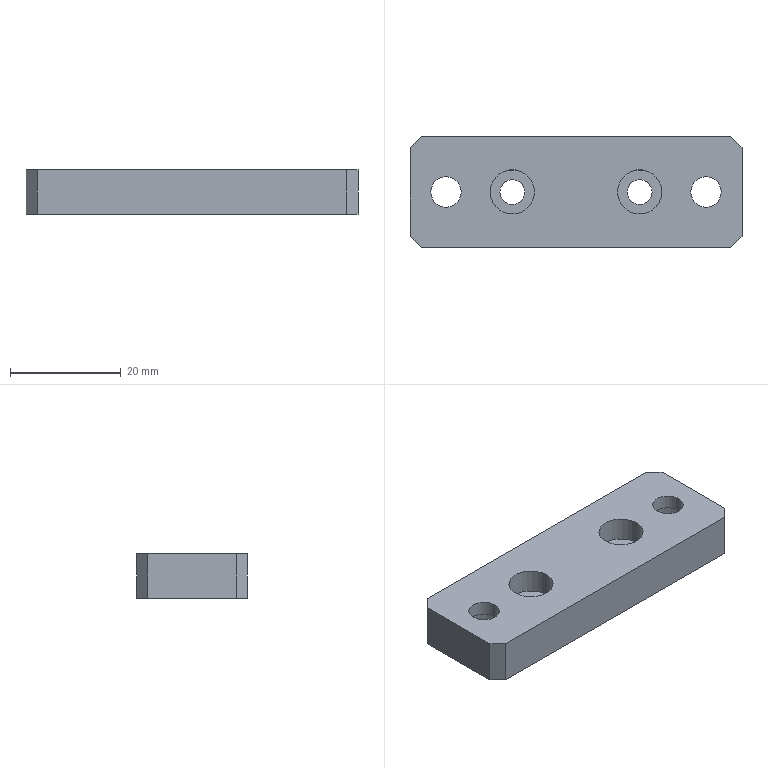Part | SolidWorks | features HoleWzd 2, Chamfer 1, Extrusion 1 | 1 solid | 30 faces | box 60 x 20 x 8 mm | volume 8007 mm3 | cylinder 16 | plane 14 | commonest cylinder face diameters 4.5 x4 5.5 x4 8 x4 10 x4
STEP:
#1=CARTESIAN_POINT('',(11.5,10.,5.4));
#2=VERTEX_POINT('',#1);
#3=CARTESIAN_POINT('',(1.5,10.,5.4));
#4=VERTEX_POINT('',#3);
#5=CARTESIAN_POINT('',(6.5,10.,5.4));
#6=DIRECTION('',(0.,0.,-1.));
#7=DIRECTION('',(-1.,0.,0.));
#8=AXIS2_PLACEMENT_3D('',#5,#6,#7);
#9=CIRCLE('',#8,5.);
#10=EDGE_CURVE('',#2,#4,#9,.T.);
#11=ORIENTED_EDGE('',*,*,#10,.F.);
#12=CARTESIAN_POINT('',(11.5,10.,0.));
#13=VERTEX_POINT('',#12);
#14=CARTESIAN_POINT('',(11.5,10.,0.));
#15=DIRECTION('',(0.,0.,-1.));
#16=VECTOR('',#15,1000.);
#17=LINE('',#14,#16);
#18=EDGE_CURVE('',#2,#13,#17,.T.);
#19=ORIENTED_EDGE('',*,*,#18,.T.);
#20=CARTESIAN_POINT('',(1.5,10.,0.));
#21=VERTEX_POINT('',#20);
#22=CARTESIAN_POINT('',(6.5,10.,0.));
#23=DIRECTION('',(0.,0.,-1.));
#24=DIRECTION('',(-1.,0.,0.));
#25=AXIS2_PLACEMENT_3D('',#22,#23,#24);
#26=CIRCLE('',#25,5.);
#27=EDGE_CURVE('',#13,#21,#26,.T.);
#28=ORIENTED_EDGE('',*,*,#27,.T.);
#29=CARTESIAN_POINT('',(1.5,10.,0.));
#30=DIRECTION('',(0.,0.,-1.));
#31=VECTOR('',#30,1000.);
#32=LINE('',#29,#31);
#33=EDGE_CURVE('',#4,#21,#32,.T.);
#34=ORIENTED_EDGE('',*,*,#33,.F.);
#35=EDGE_LOOP('',(#11,#19,#28,#34));
#36=FACE_OUTER_BOUND('',#35,.T.);
#37=CARTESIAN_POINT('',(6.5,10.,0.));
#38=DIRECTION('',(0.,0.,-1.));
#39=DIRECTION('',(-1.,0.,0.));
#40=AXIS2_PLACEMENT_3D('',#37,#38,#39);
#41=CYLINDRICAL_SURFACE('',#40,5.);
#42=ADVANCED_FACE('',(#36),#41,.F.);
#43=CARTESIAN_POINT('',(9.25,10.,8.));
#44=VERTEX_POINT('',#43);
#45=CARTESIAN_POINT('',(3.75,10.,8.));
#46=VERTEX_POINT('',#45);
#47=CARTESIAN_POINT('',(6.5,10.,8.));
#48=DIRECTION('',(0.,0.,-1.));
#49=DIRECTION('',(-1.,0.,0.));
#50=AXIS2_PLACEMENT_3D('',#47,#48,#49);
#51=CIRCLE('',#50,2.75);
#52=EDGE_CURVE('',#44,#46,#51,.T.);
#53=ORIENTED_EDGE('',*,*,#52,.F.);
#54=CARTESIAN_POINT('',(9.25,10.,5.4));
#55=VERTEX_POINT('',#54);
#56=CARTESIAN_POINT('',(9.25,10.,0.));
#57=DIRECTION('',(0.,0.,-1.));
#58=VECTOR('',#57,1000.);
#59=LINE('',#56,#58);
#60=EDGE_CURVE('',#44,#55,#59,.T.);
#61=ORIENTED_EDGE('',*,*,#60,.T.);
#62=CARTESIAN_POINT('',(3.75,10.,5.4));
#63=VERTEX_POINT('',#62);
#64=CARTESIAN_POINT('',(6.5,10.,5.4));
#65=DIRECTION('',(0.,0.,-1.));
#66=DIRECTION('',(-1.,0.,0.));
#67=AXIS2_PLACEMENT_3D('',#64,#65,#66);
#68=CIRCLE('',#67,2.75);
#69=EDGE_CURVE('',#55,#63,#68,.T.);
#70=ORIENTED_EDGE('',*,*,#69,.T.);
#71=CARTESIAN_POINT('',(3.75,10.,0.));
#72=DIRECTION('',(0.,0.,-1.));
#73=VECTOR('',#72,1000.);
#74=LINE('',#71,#73);
#75=EDGE_CURVE('',#46,#63,#74,.T.);
#76=ORIENTED_EDGE('',*,*,#75,.F.);
#77=EDGE_LOOP('',(#53,#61,#70,#76));
#78=FACE_OUTER_BOUND('',#77,.T.);
#79=CARTESIAN_POINT('',(6.5,10.,0.));
#80=DIRECTION('',(0.,0.,-1.));
#81=DIRECTION('',(-1.,0.,0.));
#82=AXIS2_PLACEMENT_3D('',#79,#80,#81);
#83=CYLINDRICAL_SURFACE('',#82,2.75);
#84=ADVANCED_FACE('',(#78),#83,.F.);
#85=CARTESIAN_POINT('',(58.5,10.,5.4));
#86=VERTEX_POINT('',#85);
#87=CARTESIAN_POINT('',(48.5,10.,5.4));
#88=VERTEX_POINT('',#87);
#89=CARTESIAN_POINT('',(53.5,10.,5.4));
#90=DIRECTION('',(0.,0.,-1.));
#91=DIRECTION('',(-1.,0.,0.));
#92=AXIS2_PLACEMENT_3D('',#89,#90,#91);
#93=CIRCLE('',#92,5.);
#94=EDGE_CURVE('',#86,#88,#93,.T.);
#95=ORIENTED_EDGE('',*,*,#94,.F.);
#96=CARTESIAN_POINT('',(58.5,10.,0.));
#97=VERTEX_POINT('',#96);
#98=CARTESIAN_POINT('',(58.5,10.,0.));
#99=DIRECTION('',(0.,0.,-1.));
#100=VECTOR('',#99,1000.);
#101=LINE('',#98,#100);
#102=EDGE_CURVE('',#86,#97,#101,.T.);
#103=ORIENTED_EDGE('',*,*,#102,.T.);
#104=CARTESIAN_POINT('',(48.5,10.,0.));
#105=VERTEX_POINT('',#104);
#106=CARTESIAN_POINT('',(53.5,10.,0.));
#107=DIRECTION('',(0.,0.,-1.));
#108=DIRECTION('',(-1.,0.,0.));
#109=AXIS2_PLACEMENT_3D('',#106,#107,#108);
#110=CIRCLE('',#109,5.);
#111=EDGE_CURVE('',#97,#105,#110,.T.);
#112=ORIENTED_EDGE('',*,*,#111,.T.);
#113=CARTESIAN_POINT('',(48.5,10.,0.));
#114=DIRECTION('',(0.,0.,-1.));
#115=VECTOR('',#114,1000.);
#116=LINE('',#113,#115);
#117=EDGE_CURVE('',#88,#105,#116,.T.);
#118=ORIENTED_EDGE('',*,*,#117,.F.);
#119=EDGE_LOOP('',(#95,#103,#112,#118));
#120=FACE_OUTER_BOUND('',#119,.T.);
#121=CARTESIAN_POINT('',(53.5,10.,0.));
#122=DIRECTION('',(0.,0.,-1.));
#123=DIRECTION('',(-1.,0.,0.));
#124=AXIS2_PLACEMENT_3D('',#121,#122,#123);
#125=CYLINDRICAL_SURFACE('',#124,5.);
#126=ADVANCED_FACE('',(#120),#125,.F.);
#127=CARTESIAN_POINT('',(56.25,10.,8.));
#128=VERTEX_POINT('',#127);
#129=CARTESIAN_POINT('',(50.75,10.,8.));
#130=VERTEX_POINT('',#129);
#131=CARTESIAN_POINT('',(53.5,10.,8.));
#132=DIRECTION('',(0.,0.,-1.));
#133=DIRECTION('',(-1.,0.,0.));
#134=AXIS2_PLACEMENT_3D('',#131,#132,#133);
#135=CIRCLE('',#134,2.75);
#136=EDGE_CURVE('',#128,#130,#135,.T.);
#137=ORIENTED_EDGE('',*,*,#136,.F.);
#138=CARTESIAN_POINT('',(56.25,10.,5.4));
#139=VERTEX_POINT('',#138);
#140=CARTESIAN_POINT('',(56.25,10.,0.));
#141=DIRECTION('',(0.,0.,-1.));
#142=VECTOR('',#141,1000.);
#143=LINE('',#140,#142);
#144=EDGE_CURVE('',#128,#139,#143,.T.);
#145=ORIENTED_EDGE('',*,*,#144,.T.);
#146=CARTESIAN_POINT('',(50.75,10.,5.4));
#147=VERTEX_POINT('',#146);
#148=CARTESIAN_POINT('',(53.5,10.,5.4));
#149=DIRECTION('',(0.,0.,-1.));
#150=DIRECTION('',(-1.,0.,0.));
#151=AXIS2_PLACEMENT_3D('',#148,#149,#150);
#152=CIRCLE('',#151,2.75);
#153=EDGE_CURVE('',#139,#147,#152,.T.);
#154=ORIENTED_EDGE('',*,*,#153,.T.);
#155=CARTESIAN_POINT('',(50.75,10.,0.));
#156=DIRECTION('',(0.,0.,-1.));
#157=VECTOR('',#156,1000.);
#158=LINE('',#155,#157);
#159=EDGE_CURVE('',#130,#147,#158,.T.);
#160=ORIENTED_EDGE('',*,*,#159,.F.);
#161=EDGE_LOOP('',(#137,#145,#154,#160));
#162=FACE_OUTER_BOUND('',#161,.T.);
#163=CARTESIAN_POINT('',(53.5,10.,0.));
#164=DIRECTION('',(0.,0.,-1.));
#165=DIRECTION('',(-1.,0.,0.));
#166=AXIS2_PLACEMENT_3D('',#163,#164,#165);
#167=CYLINDRICAL_SURFACE('',#166,2.75);
#168=ADVANCED_FACE('',(#162),#167,.F.);
#169=CARTESIAN_POINT('',(14.5,10.,3.6));
#170=VERTEX_POINT('',#169);
#171=CARTESIAN_POINT('',(22.5,10.,3.6));
#172=VERTEX_POINT('',#171);
#173=CARTESIAN_POINT('',(18.5,10.,3.6));
#174=DIRECTION('',(0.,0.,1.));
#175=DIRECTION('',(1.,0.,0.));
#176=AXIS2_PLACEMENT_3D('',#173,#174,#175);
#177=CIRCLE('',#176,4.);
#178=EDGE_CURVE('',#170,#172,#177,.T.);
#179=ORIENTED_EDGE('',*,*,#178,.F.);
#180=CARTESIAN_POINT('',(14.5,10.,8.));
#181=VERTEX_POINT('',#180);
#182=CARTESIAN_POINT('',(14.5,10.,8.));
#183=DIRECTION('',(0.,0.,1.));
#184=VECTOR('',#183,1000.);
#185=LINE('',#182,#184);
#186=EDGE_CURVE('',#170,#181,#185,.T.);
#187=ORIENTED_EDGE('',*,*,#186,.T.);
#188=CARTESIAN_POINT('',(22.5,10.,8.));
#189=VERTEX_POINT('',#188);
#190=CARTESIAN_POINT('',(18.5,10.,8.));
#191=DIRECTION('',(0.,0.,1.));
#192=DIRECTION('',(1.,0.,0.));
#193=AXIS2_PLACEMENT_3D('',#190,#191,#192);
#194=CIRCLE('',#193,4.);
#195=EDGE_CURVE('',#181,#189,#194,.T.);
#196=ORIENTED_EDGE('',*,*,#195,.T.);
#197=CARTESIAN_POINT('',(22.5,10.,8.));
#198=DIRECTION('',(0.,0.,1.));
#199=VECTOR('',#198,1000.);
#200=LINE('',#197,#199);
#201=EDGE_CURVE('',#172,#189,#200,.T.);
#202=ORIENTED_EDGE('',*,*,#201,.F.);
#203=EDGE_LOOP('',(#179,#187,#196,#202));
#204=FACE_OUTER_BOUND('',#203,.T.);
#205=CARTESIAN_POINT('',(18.5,10.,8.));
#206=DIRECTION('',(0.,0.,1.));
#207=DIRECTION('',(1.,0.,0.));
#208=AXIS2_PLACEMENT_3D('',#205,#206,#207);
#209=CYLINDRICAL_SURFACE('',#208,4.);
#210=ADVANCED_FACE('',(#204),#209,.F.);
#211=CARTESIAN_POINT('',(16.25,10.,0.));
#212=VERTEX_POINT('',#211);
#213=CARTESIAN_POINT('',(20.75,10.,0.));
#214=VERTEX_POINT('',#213);
#215=CARTESIAN_POINT('',(18.5,10.,0.));
#216=DIRECTION('',(0.,0.,1.));
#217=DIRECTION('',(1.,0.,0.));
#218=AXIS2_PLACEMENT_3D('',#215,#216,#217);
#219=CIRCLE('',#218,2.25);
#220=EDGE_CURVE('',#212,#214,#219,.T.);
#221=ORIENTED_EDGE('',*,*,#220,.F.);
#222=CARTESIAN_POINT('',(16.25,10.,3.6));
#223=VERTEX_POINT('',#222);
#224=CARTESIAN_POINT('',(16.25,10.,8.));
#225=DIRECTION('',(0.,0.,1.));
#226=VECTOR('',#225,1000.);
#227=LINE('',#224,#226);
#228=EDGE_CURVE('',#212,#223,#227,.T.);
#229=ORIENTED_EDGE('',*,*,#228,.T.);
#230=CARTESIAN_POINT('',(20.75,10.,3.6));
#231=VERTEX_POINT('',#230);
#232=CARTESIAN_POINT('',(18.5,10.,3.6));
#233=DIRECTION('',(0.,0.,1.));
#234=DIRECTION('',(1.,0.,0.));
#235=AXIS2_PLACEMENT_3D('',#232,#233,#234);
#236=CIRCLE('',#235,2.25);
#237=EDGE_CURVE('',#223,#231,#236,.T.);
#238=ORIENTED_EDGE('',*,*,#237,.T.);
#239=CARTESIAN_POINT('',(20.75,10.,8.));
#240=DIRECTION('',(0.,0.,1.));
#241=VECTOR('',#240,1000.);
#242=LINE('',#239,#241);
#243=EDGE_CURVE('',#214,#231,#242,.T.);
#244=ORIENTED_EDGE('',*,*,#243,.F.);
#245=EDGE_LOOP('',(#221,#229,#238,#244));
#246=FACE_OUTER_BOUND('',#245,.T.);
#247=CARTESIAN_POINT('',(18.5,10.,8.));
#248=DIRECTION('',(0.,0.,1.));
#249=DIRECTION('',(1.,0.,0.));
#250=AXIS2_PLACEMENT_3D('',#247,#248,#249);
#251=CYLINDRICAL_SURFACE('',#250,2.25);
#252=ADVANCED_FACE('',(#246),#251,.F.);
#253=CARTESIAN_POINT('',(37.5,10.,3.6));
#254=VERTEX_POINT('',#253);
#255=CARTESIAN_POINT('',(45.5,10.,3.6));
#256=VERTEX_POINT('',#255);
#257=CARTESIAN_POINT('',(41.5,10.,3.6));
#258=DIRECTION('',(0.,0.,1.));
#259=DIRECTION('',(1.,0.,0.));
#260=AXIS2_PLACEMENT_3D('',#257,#258,#259);
#261=CIRCLE('',#260,4.);
#262=EDGE_CURVE('',#254,#256,#261,.T.);
#263=ORIENTED_EDGE('',*,*,#262,.F.);
#264=CARTESIAN_POINT('',(37.5,10.,8.));
#265=VERTEX_POINT('',#264);
#266=CARTESIAN_POINT('',(37.5,10.,8.));
#267=DIRECTION('',(0.,0.,1.));
#268=VECTOR('',#267,1000.);
#269=LINE('',#266,#268);
#270=EDGE_CURVE('',#254,#265,#269,.T.);
#271=ORIENTED_EDGE('',*,*,#270,.T.);
#272=CARTESIAN_POINT('',(45.5,10.,8.));
#273=VERTEX_POINT('',#272);
#274=CARTESIAN_POINT('',(41.5,10.,8.));
#275=DIRECTION('',(0.,0.,1.));
#276=DIRECTION('',(1.,0.,0.));
#277=AXIS2_PLACEMENT_3D('',#274,#275,#276);
#278=CIRCLE('',#277,4.);
#279=EDGE_CURVE('',#265,#273,#278,.T.);
#280=ORIENTED_EDGE('',*,*,#279,.T.);
#281=CARTESIAN_POINT('',(45.5,10.,8.));
#282=DIRECTION('',(0.,0.,1.));
#283=VECTOR('',#282,1000.);
#284=LINE('',#281,#283);
#285=EDGE_CURVE('',#256,#273,#284,.T.);
#286=ORIENTED_EDGE('',*,*,#285,.F.);
#287=EDGE_LOOP('',(#263,#271,#280,#286));
#288=FACE_OUTER_BOUND('',#287,.T.);
#289=CARTESIAN_POINT('',(41.5,10.,8.));
#290=DIRECTION('',(0.,0.,1.));
#291=DIRECTION('',(1.,0.,0.));
#292=AXIS2_PLACEMENT_3D('',#289,#290,#291);
#293=CYLINDRICAL_SURFACE('',#292,4.);
#294=ADVANCED_FACE('',(#288),#293,.F.);
#295=CARTESIAN_POINT('',(39.25,10.,0.));
#296=VERTEX_POINT('',#295);
#297=CARTESIAN_POINT('',(43.75,10.,0.));
#298=VERTEX_POINT('',#297);
#299=CARTESIAN_POINT('',(41.5,10.,0.));
#300=DIRECTION('',(0.,0.,1.));
#301=DIRECTION('',(1.,0.,0.));
#302=AXIS2_PLACEMENT_3D('',#299,#300,#301);
#303=CIRCLE('',#302,2.25);
#304=EDGE_CURVE('',#296,#298,#303,.T.);
#305=ORIENTED_EDGE('',*,*,#304,.F.);
#306=CARTESIAN_POINT('',(39.25,10.,3.6));
#307=VERTEX_POINT('',#306);
#308=CARTESIAN_POINT('',(39.25,10.,8.));
#309=DIRECTION('',(0.,0.,1.));
#310=VECTOR('',#309,1000.);
#311=LINE('',#308,#310);
#312=EDGE_CURVE('',#296,#307,#311,.T.);
#313=ORIENTED_EDGE('',*,*,#312,.T.);
#314=CARTESIAN_POINT('',(43.75,10.,3.6));
#315=VERTEX_POINT('',#314);
#316=CARTESIAN_POINT('',(41.5,10.,3.6));
#317=DIRECTION('',(0.,0.,1.));
#318=DIRECTION('',(1.,0.,0.));
#319=AXIS2_PLACEMENT_3D('',#316,#317,#318);
#320=CIRCLE('',#319,2.25);
#321=EDGE_CURVE('',#307,#315,#320,.T.);
#322=ORIENTED_EDGE('',*,*,#321,.T.);
#323=CARTESIAN_POINT('',(43.75,10.,8.));
#324=DIRECTION('',(0.,0.,1.));
#325=VECTOR('',#324,1000.);
#326=LINE('',#323,#325);
#327=EDGE_CURVE('',#298,#315,#326,.T.);
#328=ORIENTED_EDGE('',*,*,#327,.F.);
#329=EDGE_LOOP('',(#305,#313,#322,#328));
#330=FACE_OUTER_BOUND('',#329,.T.);
#331=CARTESIAN_POINT('',(41.5,10.,8.));
#332=DIRECTION('',(0.,0.,1.));
#333=DIRECTION('',(1.,0.,0.));
#334=AXIS2_PLACEMENT_3D('',#331,#332,#333);
#335=CYLINDRICAL_SURFACE('',#334,2.25);
#336=ADVANCED_FACE('',(#330),#335,.F.);
#337=CARTESIAN_POINT('',(0.,18.,8.));
#338=VERTEX_POINT('',#337);
#339=CARTESIAN_POINT('',(0.,2.,8.));
#340=VERTEX_POINT('',#339);
#341=CARTESIAN_POINT('',(0.,0.,8.));
#342=DIRECTION('',(0.,-1.,0.));
#343=VECTOR('',#342,1000.);
#344=LINE('',#341,#343);
#345=EDGE_CURVE('',#338,#340,#344,.T.);
#346=ORIENTED_EDGE('',*,*,#345,.F.);
#347=CARTESIAN_POINT('',(0.,18.,0.));
#348=VERTEX_POINT('',#347);
#349=CARTESIAN_POINT('',(0.,18.,8.));
#350=DIRECTION('',(0.,0.,-1.));
#351=VECTOR('',#350,1000.);
#352=LINE('',#349,#351);
#353=EDGE_CURVE('',#338,#348,#352,.T.);
#354=ORIENTED_EDGE('',*,*,#353,.T.);
#355=CARTESIAN_POINT('',(0.,2.,0.));
#356=VERTEX_POINT('',#355);
#357=CARTESIAN_POINT('',(0.,0.,0.));
#358=DIRECTION('',(0.,-1.,0.));
#359=VECTOR('',#358,1000.);
#360=LINE('',#357,#359);
#361=EDGE_CURVE('',#348,#356,#360,.T.);
#362=ORIENTED_EDGE('',*,*,#361,.T.);
#363=CARTESIAN_POINT('',(0.,2.,8.));
#364=DIRECTION('',(0.,0.,1.));
#365=VECTOR('',#364,1000.);
#366=LINE('',#363,#365);
#367=EDGE_CURVE('',#356,#340,#366,.T.);
#368=ORIENTED_EDGE('',*,*,#367,.T.);
#369=EDGE_LOOP('',(#346,#354,#362,#368));
#370=FACE_OUTER_BOUND('',#369,.T.);
#371=CARTESIAN_POINT('',(0.,0.,8.));
#372=DIRECTION('',(1.,0.,0.));
#373=DIRECTION('',(0.,0.,-1.));
#374=AXIS2_PLACEMENT_3D('',#371,#372,#373);
#375=PLANE('',#374);
#376=ADVANCED_FACE('',(#370),#375,.F.);
#377=CARTESIAN_POINT('',(2.,0.,0.));
#378=VERTEX_POINT('',#377);
#379=CARTESIAN_POINT('',(58.,0.,0.));
#380=VERTEX_POINT('',#379);
#381=CARTESIAN_POINT('',(0.,0.,0.));
#382=DIRECTION('',(1.,0.,0.));
#383=VECTOR('',#382,1000.);
#384=LINE('',#381,#383);
#385=EDGE_CURVE('',#378,#380,#384,.T.);
#386=ORIENTED_EDGE('',*,*,#385,.T.);
#387=CARTESIAN_POINT('',(58.,0.,8.));
#388=VERTEX_POINT('',#387);
#389=CARTESIAN_POINT('',(58.,0.,8.));
#390=DIRECTION('',(0.,0.,1.));
#391=VECTOR('',#390,1000.);
#392=LINE('',#389,#391);
#393=EDGE_CURVE('',#380,#388,#392,.T.);
#394=ORIENTED_EDGE('',*,*,#393,.T.);
#395=CARTESIAN_POINT('',(2.,0.,8.));
#396=VERTEX_POINT('',#395);
#397=CARTESIAN_POINT('',(0.,0.,8.));
#398=DIRECTION('',(1.,0.,0.));
#399=VECTOR('',#398,1000.);
#400=LINE('',#397,#399);
#401=EDGE_CURVE('',#396,#388,#400,.T.);
#402=ORIENTED_EDGE('',*,*,#401,.F.);
#403=CARTESIAN_POINT('',(2.,0.,8.));
#404=DIRECTION('',(0.,0.,-1.));
#405=VECTOR('',#404,1000.);
#406=LINE('',#403,#405);
#407=EDGE_CURVE('',#396,#378,#406,.T.);
#408=ORIENTED_EDGE('',*,*,#407,.T.);
#409=EDGE_LOOP('',(#386,#394,#402,#408));
#410=FACE_OUTER_BOUND('',#409,.T.);
#411=CARTESIAN_POINT('',(0.,0.,8.));
#412=DIRECTION('',(0.,1.,0.));
#413=DIRECTION('',(0.,0.,1.));
#414=AXIS2_PLACEMENT_3D('',#411,#412,#413);
#415=PLANE('',#414);
#416=ADVANCED_FACE('',(#410),#415,.F.);
#417=CARTESIAN_POINT('',(60.,2.,0.));
#418=VERTEX_POINT('',#417);
#419=CARTESIAN_POINT('',(60.,18.,0.));
#420=VERTEX_POINT('',#419);
#421=CARTESIAN_POINT('',(60.,0.,0.));
#422=DIRECTION('',(0.,1.,0.));
#423=VECTOR('',#422,1000.);
#424=LINE('',#421,#423);
#425=EDGE_CURVE('',#418,#420,#424,.T.);
#426=ORIENTED_EDGE('',*,*,#425,.T.);
#427=CARTESIAN_POINT('',(60.,18.,8.));
#428=VERTEX_POINT('',#427);
#429=CARTESIAN_POINT('',(60.,18.,8.));
#430=DIRECTION('',(0.,0.,1.));
#431=VECTOR('',#430,1000.);
#432=LINE('',#429,#431);
#433=EDGE_CURVE('',#420,#428,#432,.T.);
#434=ORIENTED_EDGE('',*,*,#433,.T.);
#435=CARTESIAN_POINT('',(60.,2.,8.));
#436=VERTEX_POINT('',#435);
#437=CARTESIAN_POINT('',(60.,0.,8.));
#438=DIRECTION('',(0.,1.,0.));
#439=VECTOR('',#438,1000.);
#440=LINE('',#437,#439);
#441=EDGE_CURVE('',#436,#428,#440,.T.);
#442=ORIENTED_EDGE('',*,*,#441,.F.);
#443=CARTESIAN_POINT('',(60.,2.,8.));
#444=DIRECTION('',(0.,0.,-1.));
#445=VECTOR('',#444,1000.);
#446=LINE('',#443,#445);
#447=EDGE_CURVE('',#436,#418,#446,.T.);
#448=ORIENTED_EDGE('',*,*,#447,.T.);
#449=EDGE_LOOP('',(#426,#434,#442,#448));
#450=FACE_OUTER_BOUND('',#449,.T.);
#451=CARTESIAN_POINT('',(60.,0.,8.));
#452=DIRECTION('',(-1.,0.,0.));
#453=DIRECTION('',(0.,0.,1.));
#454=AXIS2_PLACEMENT_3D('',#451,#452,#453);
#455=PLANE('',#454);
#456=ADVANCED_FACE('',(#450),#455,.F.);
#457=CARTESIAN_POINT('',(58.,20.,8.));
#458=VERTEX_POINT('',#457);
#459=CARTESIAN_POINT('',(2.,20.,8.));
#460=VERTEX_POINT('',#459);
#461=CARTESIAN_POINT('',(0.,20.,8.));
#462=DIRECTION('',(-1.,0.,0.));
#463=VECTOR('',#462,1000.);
#464=LINE('',#461,#463);
#465=EDGE_CURVE('',#458,#460,#464,.T.);
#466=ORIENTED_EDGE('',*,*,#465,.F.);
#467=CARTESIAN_POINT('',(58.,20.,0.));
#468=VERTEX_POINT('',#467);
#469=CARTESIAN_POINT('',(58.,20.,8.));
#470=DIRECTION('',(0.,0.,-1.));
#471=VECTOR('',#470,1000.);
#472=LINE('',#469,#471);
#473=EDGE_CURVE('',#458,#468,#472,.T.);
#474=ORIENTED_EDGE('',*,*,#473,.T.);
#475=CARTESIAN_POINT('',(2.,20.,0.));
#476=VERTEX_POINT('',#475);
#477=CARTESIAN_POINT('',(0.,20.,0.));
#478=DIRECTION('',(-1.,0.,0.));
#479=VECTOR('',#478,1000.);
#480=LINE('',#477,#479);
#481=EDGE_CURVE('',#468,#476,#480,.T.);
#482=ORIENTED_EDGE('',*,*,#481,.T.);
#483=CARTESIAN_POINT('',(2.,20.,8.));
#484=DIRECTION('',(0.,0.,1.));
#485=VECTOR('',#484,1000.);
#486=LINE('',#483,#485);
#487=EDGE_CURVE('',#476,#460,#486,.T.);
#488=ORIENTED_EDGE('',*,*,#487,.T.);
#489=EDGE_LOOP('',(#466,#474,#482,#488));
#490=FACE_OUTER_BOUND('',#489,.T.);
#491=CARTESIAN_POINT('',(0.,20.,8.));
#492=DIRECTION('',(0.,-1.,0.));
#493=DIRECTION('',(0.,0.,-1.));
#494=AXIS2_PLACEMENT_3D('',#491,#492,#493);
#495=PLANE('',#494);
#496=ADVANCED_FACE('',(#490),#495,.F.);
#497=CARTESIAN_POINT('',(6.5,10.,8.));
#498=DIRECTION('',(0.,0.,-1.));
#499=DIRECTION('',(-1.,0.,0.));
#500=AXIS2_PLACEMENT_3D('',#497,#498,#499);
#501=CIRCLE('',#500,2.75);
#502=EDGE_CURVE('',#46,#44,#501,.T.);
#503=ORIENTED_EDGE('',*,*,#502,.T.);
#504=ORIENTED_EDGE('',*,*,#52,.T.);
#505=EDGE_LOOP('',(#503,#504));
#506=FACE_BOUND('',#505,.T.);
#507=CARTESIAN_POINT('',(53.5,10.,8.));
#508=DIRECTION('',(0.,0.,-1.));
#509=DIRECTION('',(-1.,0.,0.));
#510=AXIS2_PLACEMENT_3D('',#507,#508,#509);
#511=CIRCLE('',#510,2.75);
#512=EDGE_CURVE('',#130,#128,#511,.T.);
#513=ORIENTED_EDGE('',*,*,#512,.T.);
#514=ORIENTED_EDGE('',*,*,#136,.T.);
#515=EDGE_LOOP('',(#513,#514));
#516=FACE_BOUND('',#515,.T.);
#517=CARTESIAN_POINT('',(18.5,10.,8.));
#518=DIRECTION('',(0.,0.,1.));
#519=DIRECTION('',(1.,0.,0.));
#520=AXIS2_PLACEMENT_3D('',#517,#518,#519);
#521=CIRCLE('',#520,4.);
#522=EDGE_CURVE('',#189,#181,#521,.T.);
#523=ORIENTED_EDGE('',*,*,#522,.F.);
#524=ORIENTED_EDGE('',*,*,#195,.F.);
#525=EDGE_LOOP('',(#523,#524));
#526=FACE_BOUND('',#525,.T.);
#527=CARTESIAN_POINT('',(41.5,10.,8.));
#528=DIRECTION('',(0.,0.,1.));
#529=DIRECTION('',(1.,0.,0.));
#530=AXIS2_PLACEMENT_3D('',#527,#528,#529);
#531=CIRCLE('',#530,4.);
#532=EDGE_CURVE('',#273,#265,#531,.T.);
#533=ORIENTED_EDGE('',*,*,#532,.F.);
#534=ORIENTED_EDGE('',*,*,#279,.F.);
#535=EDGE_LOOP('',(#533,#534));
#536=FACE_BOUND('',#535,.T.);
#537=ORIENTED_EDGE('',*,*,#441,.T.);
#538=CARTESIAN_POINT('',(58.,20.,8.));
#539=DIRECTION('',(-0.7071,0.7071,0.));
#540=VECTOR('',#539,1000.);
#541=LINE('',#538,#540);
#542=EDGE_CURVE('',#428,#458,#541,.T.);
#543=ORIENTED_EDGE('',*,*,#542,.T.);
#544=ORIENTED_EDGE('',*,*,#465,.T.);
#545=CARTESIAN_POINT('',(0.,18.,8.));
#546=DIRECTION('',(-0.7071,-0.7071,0.));
#547=VECTOR('',#546,1000.);
#548=LINE('',#545,#547);
#549=EDGE_CURVE('',#460,#338,#548,.T.);
#550=ORIENTED_EDGE('',*,*,#549,.T.);
#551=ORIENTED_EDGE('',*,*,#345,.T.);
#552=CARTESIAN_POINT('',(2.,0.,8.));
#553=DIRECTION('',(0.7071,-0.7071,0.));
#554=VECTOR('',#553,1000.);
#555=LINE('',#552,#554);
#556=EDGE_CURVE('',#340,#396,#555,.T.);
#557=ORIENTED_EDGE('',*,*,#556,.T.);
#558=ORIENTED_EDGE('',*,*,#401,.T.);
#559=CARTESIAN_POINT('',(60.,2.,8.));
#560=DIRECTION('',(0.7071,0.7071,0.));
#561=VECTOR('',#560,1000.);
#562=LINE('',#559,#561);
#563=EDGE_CURVE('',#388,#436,#562,.T.);
#564=ORIENTED_EDGE('',*,*,#563,.T.);
#565=EDGE_LOOP('',(#537,#543,#544,#550,#551,#557,#558,#564));
#566=FACE_OUTER_BOUND('',#565,.T.);
#567=CARTESIAN_POINT('',(0.,0.,8.));
#568=DIRECTION('',(0.,0.,-1.));
#569=DIRECTION('',(-1.,0.,0.));
#570=AXIS2_PLACEMENT_3D('',#567,#568,#569);
#571=PLANE('',#570);
#572=ADVANCED_FACE('',(#506,#516,#526,#536,#566),#571,.F.);
#573=CARTESIAN_POINT('',(6.5,10.,0.));
#574=DIRECTION('',(0.,0.,-1.));
#575=DIRECTION('',(-1.,0.,0.));
#576=AXIS2_PLACEMENT_3D('',#573,#574,#575);
#577=CIRCLE('',#576,5.);
#578=EDGE_CURVE('',#21,#13,#577,.T.);
#579=ORIENTED_EDGE('',*,*,#578,.F.);
#580=ORIENTED_EDGE('',*,*,#27,.F.);
#581=EDGE_LOOP('',(#579,#580));
#582=FACE_BOUND('',#581,.T.);
#583=CARTESIAN_POINT('',(53.5,10.,0.));
#584=DIRECTION('',(0.,0.,-1.));
#585=DIRECTION('',(-1.,0.,0.));
#586=AXIS2_PLACEMENT_3D('',#583,#584,#585);
#587=CIRCLE('',#586,5.);
#588=EDGE_CURVE('',#105,#97,#587,.T.);
#589=ORIENTED_EDGE('',*,*,#588,.F.);
#590=ORIENTED_EDGE('',*,*,#111,.F.);
#591=EDGE_LOOP('',(#589,#590));
#592=FACE_BOUND('',#591,.T.);
#593=CARTESIAN_POINT('',(18.5,10.,0.));
#594=DIRECTION('',(0.,0.,1.));
#595=DIRECTION('',(1.,0.,0.));
#596=AXIS2_PLACEMENT_3D('',#593,#594,#595);
#597=CIRCLE('',#596,2.25);
#598=EDGE_CURVE('',#214,#212,#597,.T.);
#599=ORIENTED_EDGE('',*,*,#598,.T.);
#600=ORIENTED_EDGE('',*,*,#220,.T.);
#601=EDGE_LOOP('',(#599,#600));
#602=FACE_BOUND('',#601,.T.);
#603=CARTESIAN_POINT('',(41.5,10.,0.));
#604=DIRECTION('',(0.,0.,1.));
#605=DIRECTION('',(1.,0.,0.));
#606=AXIS2_PLACEMENT_3D('',#603,#604,#605);
#607=CIRCLE('',#606,2.25);
#608=EDGE_CURVE('',#298,#296,#607,.T.);
#609=ORIENTED_EDGE('',*,*,#608,.T.);
#610=ORIENTED_EDGE('',*,*,#304,.T.);
#611=EDGE_LOOP('',(#609,#610));
#612=FACE_BOUND('',#611,.T.);
#613=ORIENTED_EDGE('',*,*,#481,.F.);
#614=CARTESIAN_POINT('',(39.,39.,0.));
#615=DIRECTION('',(0.7071,-0.7071,0.));
#616=VECTOR('',#615,1000.);
#617=LINE('',#614,#616);
#618=EDGE_CURVE('',#468,#420,#617,.T.);
#619=ORIENTED_EDGE('',*,*,#618,.T.);
#620=ORIENTED_EDGE('',*,*,#425,.F.);
#621=CARTESIAN_POINT('',(29.,-29.,0.));
#622=DIRECTION('',(-0.7071,-0.7071,0.));
#623=VECTOR('',#622,1000.);
#624=LINE('',#621,#623);
#625=EDGE_CURVE('',#418,#380,#624,.T.);
#626=ORIENTED_EDGE('',*,*,#625,.T.);
#627=ORIENTED_EDGE('',*,*,#385,.F.);
#628=CARTESIAN_POINT('',(1.,1.,0.));
#629=DIRECTION('',(-0.7071,0.7071,0.));
#630=VECTOR('',#629,1000.);
#631=LINE('',#628,#630);
#632=EDGE_CURVE('',#378,#356,#631,.T.);
#633=ORIENTED_EDGE('',*,*,#632,.T.);
#634=ORIENTED_EDGE('',*,*,#361,.F.);
#635=CARTESIAN_POINT('',(-9.,9.,0.));
#636=DIRECTION('',(0.7071,0.7071,0.));
#637=VECTOR('',#636,1000.);
#638=LINE('',#635,#637);
#639=EDGE_CURVE('',#348,#476,#638,.T.);
#640=ORIENTED_EDGE('',*,*,#639,.T.);
#641=EDGE_LOOP('',(#613,#619,#620,#626,#627,#633,#634,#640));
#642=FACE_OUTER_BOUND('',#641,.T.);
#643=CARTESIAN_POINT('',(0.,0.,0.));
#644=DIRECTION('',(0.,0.,-1.));
#645=DIRECTION('',(-1.,0.,0.));
#646=AXIS2_PLACEMENT_3D('',#643,#644,#645);
#647=PLANE('',#646);
#648=ADVANCED_FACE('',(#582,#592,#602,#612,#642),#647,.T.);
#649=ORIENTED_EDGE('',*,*,#312,.F.);
#650=ORIENTED_EDGE('',*,*,#608,.F.);
#651=ORIENTED_EDGE('',*,*,#327,.T.);
#652=CARTESIAN_POINT('',(41.5,10.,3.6));
#653=DIRECTION('',(0.,0.,1.));
#654=DIRECTION('',(1.,0.,0.));
#655=AXIS2_PLACEMENT_3D('',#652,#653,#654);
#656=CIRCLE('',#655,2.25);
#657=EDGE_CURVE('',#315,#307,#656,.T.);
#658=ORIENTED_EDGE('',*,*,#657,.T.);
#659=EDGE_LOOP('',(#649,#650,#651,#658));
#660=FACE_OUTER_BOUND('',#659,.T.);
#661=CARTESIAN_POINT('',(41.5,10.,8.));
#662=DIRECTION('',(0.,0.,1.));
#663=DIRECTION('',(1.,0.,0.));
#664=AXIS2_PLACEMENT_3D('',#661,#662,#663);
#665=CYLINDRICAL_SURFACE('',#664,2.25);
#666=ADVANCED_FACE('',(#660),#665,.F.);
#667=ORIENTED_EDGE('',*,*,#657,.F.);
#668=ORIENTED_EDGE('',*,*,#321,.F.);
#669=EDGE_LOOP('',(#667,#668));
#670=FACE_BOUND('',#669,.T.);
#671=CARTESIAN_POINT('',(41.5,10.,3.6));
#672=DIRECTION('',(0.,0.,1.));
#673=DIRECTION('',(1.,0.,0.));
#674=AXIS2_PLACEMENT_3D('',#671,#672,#673);
#675=CIRCLE('',#674,4.);
#676=EDGE_CURVE('',#256,#254,#675,.T.);
#677=ORIENTED_EDGE('',*,*,#676,.T.);
#678=ORIENTED_EDGE('',*,*,#262,.T.);
#679=EDGE_LOOP('',(#677,#678));
#680=FACE_OUTER_BOUND('',#679,.T.);
#681=CARTESIAN_POINT('',(43.75,10.,3.6));
#682=DIRECTION('',(0.,0.,-1.));
#683=DIRECTION('',(-1.,0.,0.));
#684=AXIS2_PLACEMENT_3D('',#681,#682,#683);
#685=PLANE('',#684);
#686=ADVANCED_FACE('',(#670,#680),#685,.F.);
#687=ORIENTED_EDGE('',*,*,#270,.F.);
#688=ORIENTED_EDGE('',*,*,#676,.F.);
#689=ORIENTED_EDGE('',*,*,#285,.T.);
#690=ORIENTED_EDGE('',*,*,#532,.T.);
#691=EDGE_LOOP('',(#687,#688,#689,#690));
#692=FACE_OUTER_BOUND('',#691,.T.);
#693=CARTESIAN_POINT('',(41.5,10.,8.));
#694=DIRECTION('',(0.,0.,1.));
#695=DIRECTION('',(1.,0.,0.));
#696=AXIS2_PLACEMENT_3D('',#693,#694,#695);
#697=CYLINDRICAL_SURFACE('',#696,4.);
#698=ADVANCED_FACE('',(#692),#697,.F.);
#699=ORIENTED_EDGE('',*,*,#228,.F.);
#700=ORIENTED_EDGE('',*,*,#598,.F.);
#701=ORIENTED_EDGE('',*,*,#243,.T.);
#702=CARTESIAN_POINT('',(18.5,10.,3.6));
#703=DIRECTION('',(0.,0.,1.));
#704=DIRECTION('',(1.,0.,0.));
#705=AXIS2_PLACEMENT_3D('',#702,#703,#704);
#706=CIRCLE('',#705,2.25);
#707=EDGE_CURVE('',#231,#223,#706,.T.);
#708=ORIENTED_EDGE('',*,*,#707,.T.);
#709=EDGE_LOOP('',(#699,#700,#701,#708));
#710=FACE_OUTER_BOUND('',#709,.T.);
#711=CARTESIAN_POINT('',(18.5,10.,8.));
#712=DIRECTION('',(0.,0.,1.));
#713=DIRECTION('',(1.,0.,0.));
#714=AXIS2_PLACEMENT_3D('',#711,#712,#713);
#715=CYLINDRICAL_SURFACE('',#714,2.25);
#716=ADVANCED_FACE('',(#710),#715,.F.);
#717=ORIENTED_EDGE('',*,*,#707,.F.);
#718=ORIENTED_EDGE('',*,*,#237,.F.);
#719=EDGE_LOOP('',(#717,#718));
#720=FACE_BOUND('',#719,.T.);
#721=CARTESIAN_POINT('',(18.5,10.,3.6));
#722=DIRECTION('',(0.,0.,1.));
#723=DIRECTION('',(1.,0.,0.));
#724=AXIS2_PLACEMENT_3D('',#721,#722,#723);
#725=CIRCLE('',#724,4.);
#726=EDGE_CURVE('',#172,#170,#725,.T.);
#727=ORIENTED_EDGE('',*,*,#726,.T.);
#728=ORIENTED_EDGE('',*,*,#178,.T.);
#729=EDGE_LOOP('',(#727,#728));
#730=FACE_OUTER_BOUND('',#729,.T.);
#731=CARTESIAN_POINT('',(20.75,10.,3.6));
#732=DIRECTION('',(0.,0.,-1.));
#733=DIRECTION('',(-1.,0.,0.));
#734=AXIS2_PLACEMENT_3D('',#731,#732,#733);
#735=PLANE('',#734);
#736=ADVANCED_FACE('',(#720,#730),#735,.F.);
#737=ORIENTED_EDGE('',*,*,#186,.F.);
#738=ORIENTED_EDGE('',*,*,#726,.F.);
#739=ORIENTED_EDGE('',*,*,#201,.T.);
#740=ORIENTED_EDGE('',*,*,#522,.T.);
#741=EDGE_LOOP('',(#737,#738,#739,#740));
#742=FACE_OUTER_BOUND('',#741,.T.);
#743=CARTESIAN_POINT('',(18.5,10.,8.));
#744=DIRECTION('',(0.,0.,1.));
#745=DIRECTION('',(1.,0.,0.));
#746=AXIS2_PLACEMENT_3D('',#743,#744,#745);
#747=CYLINDRICAL_SURFACE('',#746,4.);
#748=ADVANCED_FACE('',(#742),#747,.F.);
#749=ORIENTED_EDGE('',*,*,#144,.F.);
#750=ORIENTED_EDGE('',*,*,#512,.F.);
#751=ORIENTED_EDGE('',*,*,#159,.T.);
#752=CARTESIAN_POINT('',(53.5,10.,5.4));
#753=DIRECTION('',(0.,0.,-1.));
#754=DIRECTION('',(-1.,0.,0.));
#755=AXIS2_PLACEMENT_3D('',#752,#753,#754);
#756=CIRCLE('',#755,2.75);
#757=EDGE_CURVE('',#147,#139,#756,.T.);
#758=ORIENTED_EDGE('',*,*,#757,.T.);
#759=EDGE_LOOP('',(#749,#750,#751,#758));
#760=FACE_OUTER_BOUND('',#759,.T.);
#761=CARTESIAN_POINT('',(53.5,10.,0.));
#762=DIRECTION('',(0.,0.,-1.));
#763=DIRECTION('',(-1.,0.,0.));
#764=AXIS2_PLACEMENT_3D('',#761,#762,#763);
#765=CYLINDRICAL_SURFACE('',#764,2.75);
#766=ADVANCED_FACE('',(#760),#765,.F.);
#767=ORIENTED_EDGE('',*,*,#757,.F.);
#768=ORIENTED_EDGE('',*,*,#153,.F.);
#769=EDGE_LOOP('',(#767,#768));
#770=FACE_BOUND('',#769,.T.);
#771=CARTESIAN_POINT('',(53.5,10.,5.4));
#772=DIRECTION('',(0.,0.,-1.));
#773=DIRECTION('',(-1.,0.,0.));
#774=AXIS2_PLACEMENT_3D('',#771,#772,#773);
#775=CIRCLE('',#774,5.);
#776=EDGE_CURVE('',#88,#86,#775,.T.);
#777=ORIENTED_EDGE('',*,*,#776,.T.);
#778=ORIENTED_EDGE('',*,*,#94,.T.);
#779=EDGE_LOOP('',(#777,#778));
#780=FACE_OUTER_BOUND('',#779,.T.);
#781=CARTESIAN_POINT('',(56.25,10.,5.4));
#782=DIRECTION('',(0.,0.,1.));
#783=DIRECTION('',(1.,0.,0.));
#784=AXIS2_PLACEMENT_3D('',#781,#782,#783);
#785=PLANE('',#784);
#786=ADVANCED_FACE('',(#770,#780),#785,.F.);
#787=ORIENTED_EDGE('',*,*,#102,.F.);
#788=ORIENTED_EDGE('',*,*,#776,.F.);
#789=ORIENTED_EDGE('',*,*,#117,.T.);
#790=ORIENTED_EDGE('',*,*,#588,.T.);
#791=EDGE_LOOP('',(#787,#788,#789,#790));
#792=FACE_OUTER_BOUND('',#791,.T.);
#793=CARTESIAN_POINT('',(53.5,10.,0.));
#794=DIRECTION('',(0.,0.,-1.));
#795=DIRECTION('',(-1.,0.,0.));
#796=AXIS2_PLACEMENT_3D('',#793,#794,#795);
#797=CYLINDRICAL_SURFACE('',#796,5.);
#798=ADVANCED_FACE('',(#792),#797,.F.);
#799=ORIENTED_EDGE('',*,*,#60,.F.);
#800=ORIENTED_EDGE('',*,*,#502,.F.);
#801=ORIENTED_EDGE('',*,*,#75,.T.);
#802=CARTESIAN_POINT('',(6.5,10.,5.4));
#803=DIRECTION('',(0.,0.,-1.));
#804=DIRECTION('',(-1.,0.,0.));
#805=AXIS2_PLACEMENT_3D('',#802,#803,#804);
#806=CIRCLE('',#805,2.75);
#807=EDGE_CURVE('',#63,#55,#806,.T.);
#808=ORIENTED_EDGE('',*,*,#807,.T.);
#809=EDGE_LOOP('',(#799,#800,#801,#808));
#810=FACE_OUTER_BOUND('',#809,.T.);
#811=CARTESIAN_POINT('',(6.5,10.,0.));
#812=DIRECTION('',(0.,0.,-1.));
#813=DIRECTION('',(-1.,0.,0.));
#814=AXIS2_PLACEMENT_3D('',#811,#812,#813);
#815=CYLINDRICAL_SURFACE('',#814,2.75);
#816=ADVANCED_FACE('',(#810),#815,.F.);
#817=ORIENTED_EDGE('',*,*,#807,.F.);
#818=ORIENTED_EDGE('',*,*,#69,.F.);
#819=EDGE_LOOP('',(#817,#818));
#820=FACE_BOUND('',#819,.T.);
#821=CARTESIAN_POINT('',(6.5,10.,5.4));
#822=DIRECTION('',(0.,0.,-1.));
#823=DIRECTION('',(-1.,0.,0.));
#824=AXIS2_PLACEMENT_3D('',#821,#822,#823);
#825=CIRCLE('',#824,5.);
#826=EDGE_CURVE('',#4,#2,#825,.T.);
#827=ORIENTED_EDGE('',*,*,#826,.T.);
#828=ORIENTED_EDGE('',*,*,#10,.T.);
#829=EDGE_LOOP('',(#827,#828));
#830=FACE_OUTER_BOUND('',#829,.T.);
#831=CARTESIAN_POINT('',(9.25,10.,5.4));
#832=DIRECTION('',(0.,0.,1.));
#833=DIRECTION('',(1.,0.,0.));
#834=AXIS2_PLACEMENT_3D('',#831,#832,#833);
#835=PLANE('',#834);
#836=ADVANCED_FACE('',(#820,#830),#835,.F.);
#837=ORIENTED_EDGE('',*,*,#18,.F.);
#838=ORIENTED_EDGE('',*,*,#826,.F.);
#839=ORIENTED_EDGE('',*,*,#33,.T.);
#840=ORIENTED_EDGE('',*,*,#578,.T.);
#841=EDGE_LOOP('',(#837,#838,#839,#840));
#842=FACE_OUTER_BOUND('',#841,.T.);
#843=CARTESIAN_POINT('',(6.5,10.,0.));
#844=DIRECTION('',(0.,0.,-1.));
#845=DIRECTION('',(-1.,0.,0.));
#846=AXIS2_PLACEMENT_3D('',#843,#844,#845);
#847=CYLINDRICAL_SURFACE('',#846,5.);
#848=ADVANCED_FACE('',(#842),#847,.F.);
#849=ORIENTED_EDGE('',*,*,#542,.F.);
#850=ORIENTED_EDGE('',*,*,#433,.F.);
#851=ORIENTED_EDGE('',*,*,#618,.F.);
#852=ORIENTED_EDGE('',*,*,#473,.F.);
#853=EDGE_LOOP('',(#849,#850,#851,#852));
#854=FACE_OUTER_BOUND('',#853,.T.);
#855=CARTESIAN_POINT('',(58.,20.,8.));
#856=DIRECTION('',(-0.7071,-0.7071,0.));
#857=DIRECTION('',(0.,0.,-1.));
#858=AXIS2_PLACEMENT_3D('',#855,#856,#857);
#859=PLANE('',#858);
#860=ADVANCED_FACE('',(#854),#859,.F.);
#861=ORIENTED_EDGE('',*,*,#563,.F.);
#862=ORIENTED_EDGE('',*,*,#393,.F.);
#863=ORIENTED_EDGE('',*,*,#625,.F.);
#864=ORIENTED_EDGE('',*,*,#447,.F.);
#865=EDGE_LOOP('',(#861,#862,#863,#864));
#866=FACE_OUTER_BOUND('',#865,.T.);
#867=CARTESIAN_POINT('',(60.,2.,8.));
#868=DIRECTION('',(-0.7071,0.7071,0.));
#869=DIRECTION('',(0.,0.,-1.));
#870=AXIS2_PLACEMENT_3D('',#867,#868,#869);
#871=PLANE('',#870);
#872=ADVANCED_FACE('',(#866),#871,.F.);
#873=ORIENTED_EDGE('',*,*,#549,.F.);
#874=ORIENTED_EDGE('',*,*,#487,.F.);
#875=ORIENTED_EDGE('',*,*,#639,.F.);
#876=ORIENTED_EDGE('',*,*,#353,.F.);
#877=EDGE_LOOP('',(#873,#874,#875,#876));
#878=FACE_OUTER_BOUND('',#877,.T.);
#879=CARTESIAN_POINT('',(0.,18.,8.));
#880=DIRECTION('',(0.7071,-0.7071,0.));
#881=DIRECTION('',(0.,0.,-1.));
#882=AXIS2_PLACEMENT_3D('',#879,#880,#881);
#883=PLANE('',#882);
#884=ADVANCED_FACE('',(#878),#883,.F.);
#885=ORIENTED_EDGE('',*,*,#556,.F.);
#886=ORIENTED_EDGE('',*,*,#367,.F.);
#887=ORIENTED_EDGE('',*,*,#632,.F.);
#888=ORIENTED_EDGE('',*,*,#407,.F.);
#889=EDGE_LOOP('',(#885,#886,#887,#888));
#890=FACE_OUTER_BOUND('',#889,.T.);
#891=CARTESIAN_POINT('',(2.,0.,8.));
#892=DIRECTION('',(0.7071,0.7071,0.));
#893=DIRECTION('',(0.,0.,-1.));
#894=AXIS2_PLACEMENT_3D('',#891,#892,#893);
#895=PLANE('',#894);
#896=ADVANCED_FACE('',(#890),#895,.F.);
#897=CLOSED_SHELL('',(#42,#84,#126,#168,#210,#252,#294,#336,#376,#416,#456,#496,#572,#648,#666,#686,#698,#716,#736,#748,#766,#786,#798,#816,#836,#848,#860,#872,#884,#896));
#898=MANIFOLD_SOLID_BREP('',#897);
#899=CARTESIAN_POINT('',(0.,0.,0.));
#900=DIRECTION('',(0.,0.,1.));
#901=DIRECTION('',(1.,0.,0.));
#902=AXIS2_PLACEMENT_3D('',#899,#900,#901);
#903=(LENGTH_UNIT()NAMED_UNIT(*)SI_UNIT(.MILLI.,.METRE.));
#904=UNCERTAINTY_MEASURE_WITH_UNIT(LENGTH_MEASURE(0.00001),#903,'','');
#905=(NAMED_UNIT(*)PLANE_ANGLE_UNIT()SI_UNIT($,.RADIAN.));
#906=(NAMED_UNIT(*)SI_UNIT($,.STERADIAN.)SOLID_ANGLE_UNIT());
#907=(GEOMETRIC_REPRESENTATION_CONTEXT(3)GLOBAL_UNCERTAINTY_ASSIGNED_CONTEXT((#904))GLOBAL_UNIT_ASSIGNED_CONTEXT((#903,#905,#906))REPRESENTATION_CONTEXT('',''));
#908=ADVANCED_BREP_SHAPE_REPRESENTATION('',(#898,#902),#907);